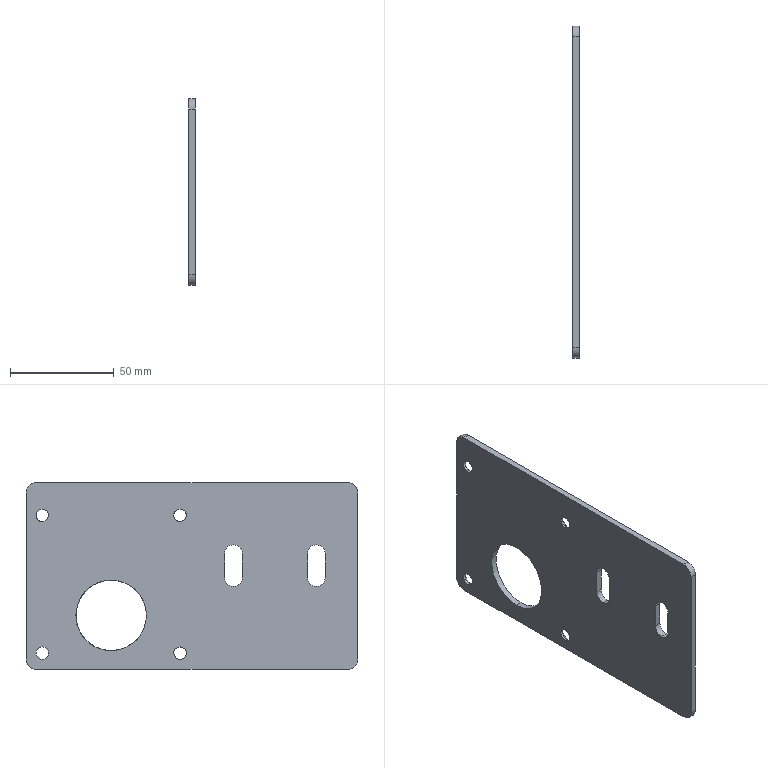Part | STEP file | 101000007723 | 1 solid | 40 faces | box 3 x 160 x 90 mm | volume 38961 mm3 | cylinder 22 | plane 10 | cone 8 | commonest cylinder face diameters 6 x8 8.5 x8 10 x4 34 x2